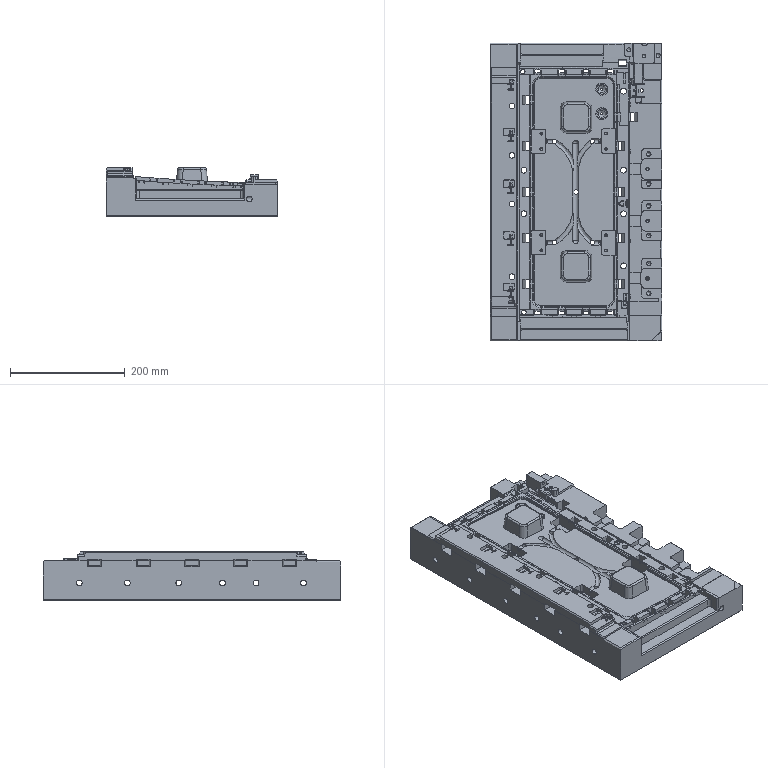Part | STEP file | solid 205 | 1 solid | 1566 faces | box 300 x 520 x 85 mm | volume 8735369 mm3 | plane 816 | cylinder 419 | spline 224 | cone 69 | torus 20 | other 14 | sphere 4 | commonest cylinder face diameters 1.004 x58 6922 x51 10 x44 1.005 x33 8 x33 4 x25